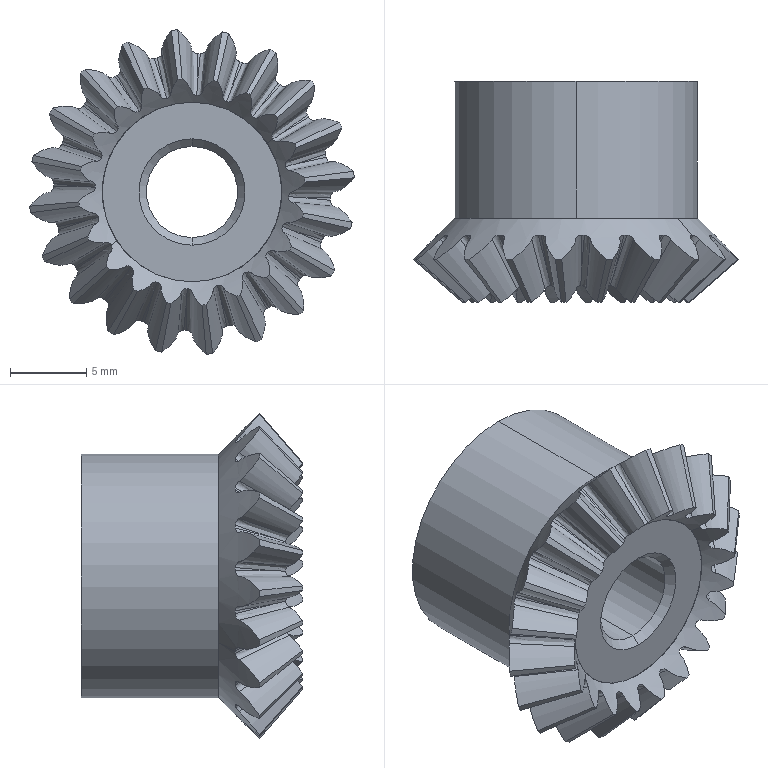Part | SolidWorks | features BaseBody 2 | 2 solids | 140 faces | box 21.332 x 14.53 x 21.332 mm | volume 2489 mm3 | spline 100 | cone 28 | cylinder 8 | plane 4 | commonest cylinder face diameters 11.8 x4 6 x2 16 x2